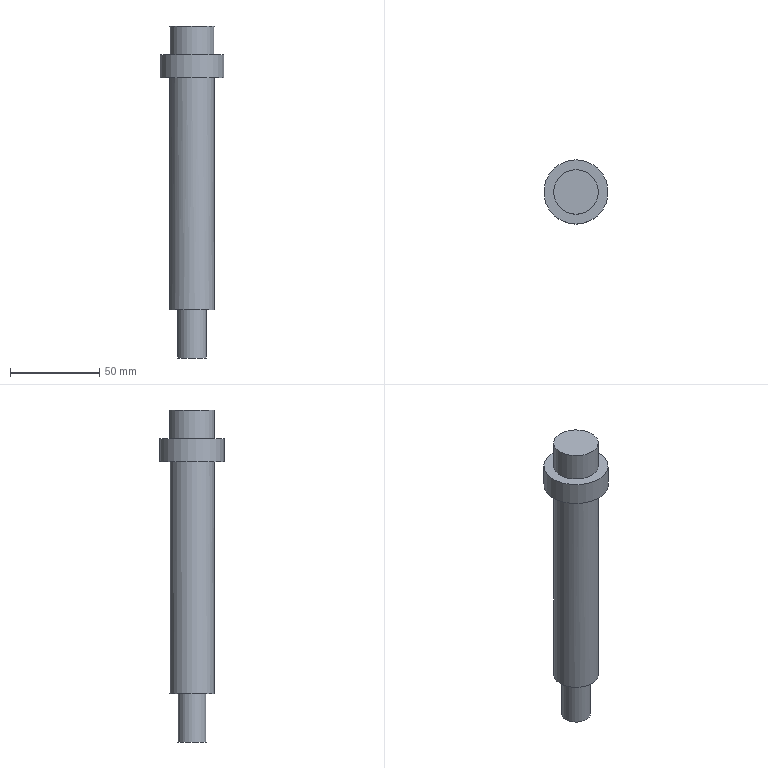Part | NX | features solid 2 | 1 solid | 9 faces | box 36 x 36 x 186 mm | volume 90329 mm3 | plane 5 | cylinder 4 | commonest cylinder face diameters 25 x2 16 x1 36 x1
STEP:
#1=CARTESIAN_POINT('',(-403.,-165.,50.));
#2=VERTEX_POINT('',#1);
#3=CARTESIAN_POINT('',(-395.,-165.,50.));
#4=DIRECTION('',(0.,0.,-1.));
#5=DIRECTION('',(-1.,0.,0.));
#6=AXIS2_PLACEMENT_3D('',#3,#4,#5);
#7=CIRCLE('',#6,8.);
#8=EDGE_CURVE('',#2,#2,#7,.T.);
#9=ORIENTED_EDGE('',*,*,#8,.F.);
#10=EDGE_LOOP('',(#9));
#11=FACE_BOUND('',#10,.T.);
#12=CARTESIAN_POINT('',(-407.5,-165.,50.));
#13=VERTEX_POINT('',#12);
#14=CARTESIAN_POINT('',(-395.,-165.,50.));
#15=DIRECTION('',(0.,0.,-1.));
#16=DIRECTION('',(-1.,0.,0.));
#17=AXIS2_PLACEMENT_3D('',#14,#15,#16);
#18=CIRCLE('',#17,12.5);
#19=EDGE_CURVE('',#13,#13,#18,.F.);
#20=ORIENTED_EDGE('',*,*,#19,.F.);
#21=EDGE_LOOP('',(#20));
#22=FACE_BOUND('',#21,.T.);
#23=CARTESIAN_POINT('',(-395.,-165.,50.));
#24=DIRECTION('',(0.,0.,-1.));
#25=DIRECTION('',(0.,-1.,0.));
#26=AXIS2_PLACEMENT_3D('',#23,#24,#25);
#27=PLANE('',#26);
#28=ADVANCED_FACE('',(#11,#22),#27,.T.);
#29=CARTESIAN_POINT('',(-395.,-177.5,180.));
#30=VERTEX_POINT('',#29);
#31=CARTESIAN_POINT('',(-395.,-165.,180.));
#32=DIRECTION('',(0.,0.,-1.));
#33=DIRECTION('',(0.,-1.,0.));
#34=AXIS2_PLACEMENT_3D('',#31,#32,#33);
#35=CIRCLE('',#34,12.5);
#36=EDGE_CURVE('',#30,#30,#35,.F.);
#37=ORIENTED_EDGE('',*,*,#36,.F.);
#38=EDGE_LOOP('',(#37));
#39=FACE_BOUND('',#38,.T.);
#40=ORIENTED_EDGE('',*,*,#19,.T.);
#41=EDGE_LOOP('',(#40));
#42=FACE_BOUND('',#41,.T.);
#43=CARTESIAN_POINT('',(-395.,-165.,-60.));
#44=DIRECTION('',(0.,0.,1.));
#45=DIRECTION('',(0.,1.,0.));
#46=AXIS2_PLACEMENT_3D('',#43,#44,#45);
#47=CYLINDRICAL_SURFACE('',#46,12.5);
#48=ADVANCED_FACE('',(#39,#42),#47,.T.);
#49=CARTESIAN_POINT('',(-403.,-165.,23.));
#50=VERTEX_POINT('',#49);
#51=CARTESIAN_POINT('',(-395.,-165.,23.));
#52=DIRECTION('',(0.,0.,-1.));
#53=DIRECTION('',(-1.,0.,0.));
#54=AXIS2_PLACEMENT_3D('',#51,#52,#53);
#55=CIRCLE('',#54,8.);
#56=EDGE_CURVE('',#50,#50,#55,.F.);
#57=ORIENTED_EDGE('',*,*,#56,.F.);
#58=EDGE_LOOP('',(#57));
#59=FACE_BOUND('',#58,.T.);
#60=CARTESIAN_POINT('',(-395.,-165.,23.));
#61=DIRECTION('',(0.,0.,-1.));
#62=DIRECTION('',(0.,-1.,0.));
#63=AXIS2_PLACEMENT_3D('',#60,#61,#62);
#64=PLANE('',#63);
#65=ADVANCED_FACE('',(#59),#64,.T.);
#66=ORIENTED_EDGE('',*,*,#56,.T.);
#67=EDGE_LOOP('',(#66));
#68=FACE_BOUND('',#67,.T.);
#69=ORIENTED_EDGE('',*,*,#8,.T.);
#70=EDGE_LOOP('',(#69));
#71=FACE_BOUND('',#70,.T.);
#72=CARTESIAN_POINT('',(-395.,-165.,-60.));
#73=DIRECTION('',(0.,0.,-1.));
#74=DIRECTION('',(0.,-1.,0.));
#75=AXIS2_PLACEMENT_3D('',#72,#73,#74);
#76=CYLINDRICAL_SURFACE('',#75,8.);
#77=ADVANCED_FACE('',(#68,#71),#76,.T.);
#78=CARTESIAN_POINT('',(-395.,-152.5,193.));
#79=VERTEX_POINT('',#78);
#80=CARTESIAN_POINT('',(-395.,-165.,193.));
#81=DIRECTION('',(0.,0.,1.));
#82=DIRECTION('',(0.,1.,0.));
#83=AXIS2_PLACEMENT_3D('',#80,#81,#82);
#84=CIRCLE('',#83,12.5);
#85=EDGE_CURVE('',#79,#79,#84,.T.);
#86=ORIENTED_EDGE('',*,*,#85,.F.);
#87=EDGE_LOOP('',(#86));
#88=FACE_BOUND('',#87,.T.);
#89=CARTESIAN_POINT('',(-395.,-183.,193.));
#90=VERTEX_POINT('',#89);
#91=CARTESIAN_POINT('',(-395.,-165.,193.));
#92=DIRECTION('',(0.,0.,-1.));
#93=DIRECTION('',(0.,-1.,0.));
#94=AXIS2_PLACEMENT_3D('',#91,#92,#93);
#95=CIRCLE('',#94,18.);
#96=EDGE_CURVE('',#90,#90,#95,.T.);
#97=ORIENTED_EDGE('',*,*,#96,.F.);
#98=EDGE_LOOP('',(#97));
#99=FACE_BOUND('',#98,.T.);
#100=CARTESIAN_POINT('',(-395.,-165.,193.));
#101=DIRECTION('',(0.,0.,1.));
#102=DIRECTION('',(0.,1.,0.));
#103=AXIS2_PLACEMENT_3D('',#100,#101,#102);
#104=PLANE('',#103);
#105=ADVANCED_FACE('',(#88,#99),#104,.T.);
#106=ORIENTED_EDGE('',*,*,#36,.T.);
#107=EDGE_LOOP('',(#106));
#108=FACE_BOUND('',#107,.T.);
#109=CARTESIAN_POINT('',(-395.,-147.,180.));
#110=VERTEX_POINT('',#109);
#111=CARTESIAN_POINT('',(-395.,-165.,180.));
#112=DIRECTION('',(0.,0.,1.));
#113=DIRECTION('',(0.,1.,0.));
#114=AXIS2_PLACEMENT_3D('',#111,#112,#113);
#115=CIRCLE('',#114,18.);
#116=EDGE_CURVE('',#110,#110,#115,.T.);
#117=ORIENTED_EDGE('',*,*,#116,.F.);
#118=EDGE_LOOP('',(#117));
#119=FACE_BOUND('',#118,.T.);
#120=CARTESIAN_POINT('',(-395.,-165.,180.));
#121=DIRECTION('',(0.,0.,-1.));
#122=DIRECTION('',(0.,-1.,0.));
#123=AXIS2_PLACEMENT_3D('',#120,#121,#122);
#124=PLANE('',#123);
#125=ADVANCED_FACE('',(#108,#119),#124,.T.);
#126=ORIENTED_EDGE('',*,*,#96,.T.);
#127=EDGE_LOOP('',(#126));
#128=FACE_BOUND('',#127,.T.);
#129=ORIENTED_EDGE('',*,*,#116,.T.);
#130=EDGE_LOOP('',(#129));
#131=FACE_BOUND('',#130,.T.);
#132=CARTESIAN_POINT('',(-395.,-165.,180.));
#133=DIRECTION('',(0.,0.,1.));
#134=DIRECTION('',(0.,1.,0.));
#135=AXIS2_PLACEMENT_3D('',#132,#133,#134);
#136=CYLINDRICAL_SURFACE('',#135,18.);
#137=ADVANCED_FACE('',(#128,#131),#136,.T.);
#138=CARTESIAN_POINT('',(-395.,-177.5,209.));
#139=VERTEX_POINT('',#138);
#140=CARTESIAN_POINT('',(-395.,-165.,209.));
#141=DIRECTION('',(0.,0.,-1.));
#142=DIRECTION('',(0.,-1.,0.));
#143=AXIS2_PLACEMENT_3D('',#140,#141,#142);
#144=CIRCLE('',#143,12.5);
#145=EDGE_CURVE('',#139,#139,#144,.T.);
#146=ORIENTED_EDGE('',*,*,#145,.F.);
#147=EDGE_LOOP('',(#146));
#148=FACE_BOUND('',#147,.T.);
#149=CARTESIAN_POINT('',(-395.,-165.,209.));
#150=DIRECTION('',(0.,0.,1.));
#151=DIRECTION('',(0.,1.,0.));
#152=AXIS2_PLACEMENT_3D('',#149,#150,#151);
#153=PLANE('',#152);
#154=ADVANCED_FACE('',(#148),#153,.T.);
#155=ORIENTED_EDGE('',*,*,#145,.T.);
#156=EDGE_LOOP('',(#155));
#157=FACE_BOUND('',#156,.T.);
#158=ORIENTED_EDGE('',*,*,#85,.T.);
#159=EDGE_LOOP('',(#158));
#160=FACE_BOUND('',#159,.T.);
#161=CARTESIAN_POINT('',(-395.,-165.,193.));
#162=DIRECTION('',(0.,0.,1.));
#163=DIRECTION('',(0.,1.,0.));
#164=AXIS2_PLACEMENT_3D('',#161,#162,#163);
#165=CYLINDRICAL_SURFACE('',#164,12.5);
#166=ADVANCED_FACE('',(#157,#160),#165,.T.);
#167=CLOSED_SHELL('',(#28,#48,#65,#77,#105,#125,#137,#154,#166));
#168=MANIFOLD_SOLID_BREP('',#167);
#169=(LENGTH_UNIT()NAMED_UNIT(*)SI_UNIT(.MILLI.,.METRE.));
#170=UNCERTAINTY_MEASURE_WITH_UNIT(LENGTH_MEASURE(0.00001),#169,'','');
#171=(NAMED_UNIT(*)PLANE_ANGLE_UNIT()SI_UNIT($,.RADIAN.));
#172=(NAMED_UNIT(*)SI_UNIT($,.STERADIAN.)SOLID_ANGLE_UNIT());
#173=(GEOMETRIC_REPRESENTATION_CONTEXT(3)GLOBAL_UNCERTAINTY_ASSIGNED_CONTEXT((#170))GLOBAL_UNIT_ASSIGNED_CONTEXT((#169,#171,#172))REPRESENTATION_CONTEXT('',''));
#174=ADVANCED_BREP_SHAPE_REPRESENTATION('',(#168),#173);